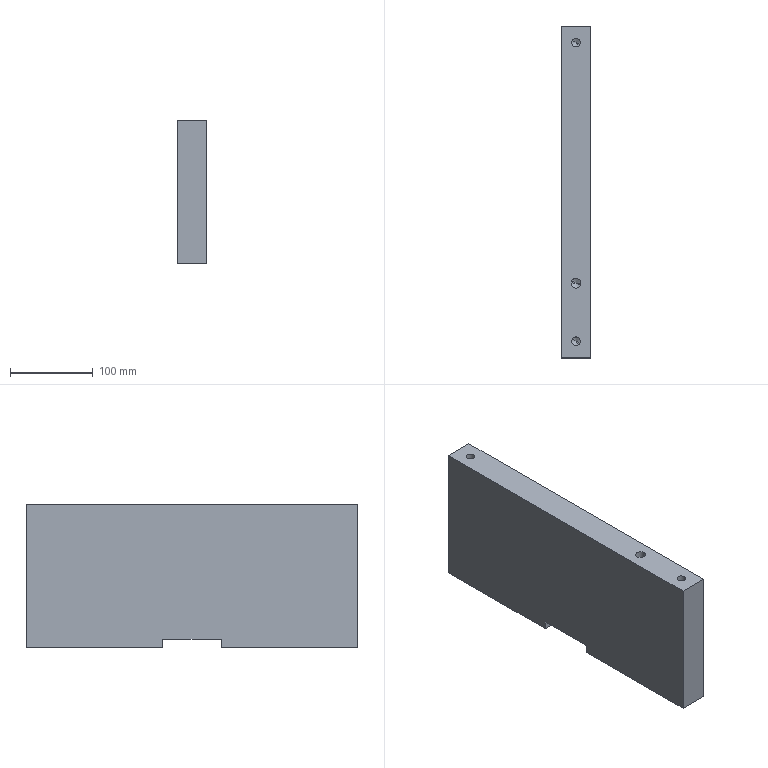Part | CATIA | 1 solid | 42 faces | box 35 x 400 x 173 mm | volume 2372229 mm3 | cone 16 | cylinder 16 | plane 10 | commonest cylinder face diameters 10.2 x10 12 x6
STEP:
#1=CARTESIAN_POINT('',(17.5,200.,-102.));
#2=VERTEX_POINT('',#1);
#3=CARTESIAN_POINT('',(17.5,200.,-275.));
#4=VERTEX_POINT('',#3);
#5=CARTESIAN_POINT('',(17.5,200.,-188.5));
#6=DIRECTION('',(0.,0.,-1.));
#7=VECTOR('',#6,1.);
#8=LINE('',#5,#7);
#9=EDGE_CURVE('',#2,#4,#8,.T.);
#10=ORIENTED_EDGE('',*,*,#9,.T.);
#11=CARTESIAN_POINT('',(-17.5,200.,-275.));
#12=VERTEX_POINT('',#11);
#13=CARTESIAN_POINT('',(0.,200.,-275.));
#14=DIRECTION('',(1.,0.,0.));
#15=VECTOR('',#14,1.);
#16=LINE('',#13,#15);
#17=EDGE_CURVE('',#4,#12,#16,.F.);
#18=ORIENTED_EDGE('',*,*,#17,.T.);
#19=CARTESIAN_POINT('',(-17.5,200.,-102.));
#20=VERTEX_POINT('',#19);
#21=CARTESIAN_POINT('',(-17.5,200.,-188.5));
#22=DIRECTION('',(0.,0.,-1.));
#23=VECTOR('',#22,1.);
#24=LINE('',#21,#23);
#25=EDGE_CURVE('',#20,#12,#24,.T.);
#26=ORIENTED_EDGE('',*,*,#25,.F.);
#27=CARTESIAN_POINT('',(0.,200.,-102.));
#28=DIRECTION('',(1.,0.,0.));
#29=VECTOR('',#28,1.);
#30=LINE('',#27,#29);
#31=EDGE_CURVE('',#20,#2,#30,.T.);
#32=ORIENTED_EDGE('',*,*,#31,.T.);
#33=EDGE_LOOP('',(#10,#18,#26,#32));
#34=FACE_OUTER_BOUND('',#33,.T.);
#35=CARTESIAN_POINT('',(-17.5,200.,0.));
#36=DIRECTION('',(0.,1.,0.));
#37=DIRECTION('',(1.,0.,0.));
#38=AXIS2_PLACEMENT_3D('',#35,#36,#37);
#39=PLANE('',#38);
#40=ADVANCED_FACE('',(#34),#39,.T.);
#41=CARTESIAN_POINT('',(-17.5,-200.,-102.));
#42=VERTEX_POINT('',#41);
#43=CARTESIAN_POINT('',(-17.5,-200.,-275.));
#44=VERTEX_POINT('',#43);
#45=CARTESIAN_POINT('',(-17.5,-200.,-188.5));
#46=DIRECTION('',(0.,0.,-1.));
#47=VECTOR('',#46,1.);
#48=LINE('',#45,#47);
#49=EDGE_CURVE('',#42,#44,#48,.T.);
#50=ORIENTED_EDGE('',*,*,#49,.T.);
#51=CARTESIAN_POINT('',(17.5,-200.,-275.));
#52=VERTEX_POINT('',#51);
#53=CARTESIAN_POINT('',(0.,-200.,-275.));
#54=DIRECTION('',(-1.,0.,0.));
#55=VECTOR('',#54,1.);
#56=LINE('',#53,#55);
#57=EDGE_CURVE('',#44,#52,#56,.F.);
#58=ORIENTED_EDGE('',*,*,#57,.T.);
#59=CARTESIAN_POINT('',(17.5,-200.,-102.));
#60=VERTEX_POINT('',#59);
#61=CARTESIAN_POINT('',(17.5,-200.,-188.5));
#62=DIRECTION('',(0.,0.,-1.));
#63=VECTOR('',#62,1.);
#64=LINE('',#61,#63);
#65=EDGE_CURVE('',#60,#52,#64,.T.);
#66=ORIENTED_EDGE('',*,*,#65,.F.);
#67=CARTESIAN_POINT('',(0.,-200.,-102.));
#68=DIRECTION('',(-1.,0.,0.));
#69=VECTOR('',#68,1.);
#70=LINE('',#67,#69);
#71=EDGE_CURVE('',#60,#42,#70,.T.);
#72=ORIENTED_EDGE('',*,*,#71,.T.);
#73=EDGE_LOOP('',(#50,#58,#66,#72));
#74=FACE_OUTER_BOUND('',#73,.T.);
#75=CARTESIAN_POINT('',(17.5,-200.,0.));
#76=DIRECTION('',(0.,-1.,0.));
#77=DIRECTION('',(-1.,0.,0.));
#78=AXIS2_PLACEMENT_3D('',#75,#76,#77);
#79=PLANE('',#78);
#80=ADVANCED_FACE('',(#74),#79,.T.);
#81=CARTESIAN_POINT('',(-17.5,35.,-275.));
#82=VERTEX_POINT('',#81);
#83=CARTESIAN_POINT('',(-17.5,35.,-265.));
#84=VERTEX_POINT('',#83);
#85=CARTESIAN_POINT('',(-17.5,35.,-270.));
#86=DIRECTION('',(0.,0.,1.));
#87=VECTOR('',#86,1.);
#88=LINE('',#85,#87);
#89=EDGE_CURVE('',#82,#84,#88,.T.);
#90=ORIENTED_EDGE('',*,*,#89,.T.);
#91=CARTESIAN_POINT('',(-17.5,-35.,-265.));
#92=VERTEX_POINT('',#91);
#93=CARTESIAN_POINT('',(-17.5,0.,-265.));
#94=DIRECTION('',(0.,1.,0.));
#95=VECTOR('',#94,1.);
#96=LINE('',#93,#95);
#97=EDGE_CURVE('',#92,#84,#96,.T.);
#98=ORIENTED_EDGE('',*,*,#97,.F.);
#99=CARTESIAN_POINT('',(-17.5,-35.,-275.));
#100=VERTEX_POINT('',#99);
#101=CARTESIAN_POINT('',(-17.5,-35.,-270.));
#102=DIRECTION('',(0.,0.,1.));
#103=VECTOR('',#102,1.);
#104=LINE('',#101,#103);
#105=EDGE_CURVE('',#100,#92,#104,.T.);
#106=ORIENTED_EDGE('',*,*,#105,.F.);
#107=CARTESIAN_POINT('',(-17.5,-117.5,-275.));
#108=DIRECTION('',(0.,-1.,0.));
#109=VECTOR('',#108,1.);
#110=LINE('',#107,#109);
#111=EDGE_CURVE('',#100,#44,#110,.T.);
#112=ORIENTED_EDGE('',*,*,#111,.T.);
#113=ORIENTED_EDGE('',*,*,#49,.F.);
#114=CARTESIAN_POINT('',(-17.5,0.,-102.));
#115=DIRECTION('',(0.,-1.,0.));
#116=VECTOR('',#115,1.);
#117=LINE('',#114,#116);
#118=EDGE_CURVE('',#20,#42,#117,.T.);
#119=ORIENTED_EDGE('',*,*,#118,.F.);
#120=ORIENTED_EDGE('',*,*,#25,.T.);
#121=CARTESIAN_POINT('',(-17.5,117.5,-275.));
#122=DIRECTION('',(0.,-1.,0.));
#123=VECTOR('',#122,1.);
#124=LINE('',#121,#123);
#125=EDGE_CURVE('',#12,#82,#124,.T.);
#126=ORIENTED_EDGE('',*,*,#125,.T.);
#127=EDGE_LOOP('',(#90,#98,#106,#112,#113,#119,#120,#126));
#128=FACE_OUTER_BOUND('',#127,.T.);
#129=CARTESIAN_POINT('',(-17.5,200.,0.));
#130=DIRECTION('',(1.,0.,0.));
#131=DIRECTION('',(0.,-1.,0.));
#132=AXIS2_PLACEMENT_3D('',#129,#130,#131);
#133=PLANE('',#132);
#134=ADVANCED_FACE('',(#128),#133,.F.);
#135=CARTESIAN_POINT('',(17.5,-35.,-275.));
#136=VERTEX_POINT('',#135);
#137=CARTESIAN_POINT('',(17.5,-35.,-265.));
#138=VERTEX_POINT('',#137);
#139=CARTESIAN_POINT('',(17.5,-35.,-270.));
#140=DIRECTION('',(0.,0.,1.));
#141=VECTOR('',#140,1.);
#142=LINE('',#139,#141);
#143=EDGE_CURVE('',#136,#138,#142,.T.);
#144=ORIENTED_EDGE('',*,*,#143,.T.);
#145=CARTESIAN_POINT('',(17.5,35.,-265.));
#146=VERTEX_POINT('',#145);
#147=CARTESIAN_POINT('',(17.5,0.,-265.));
#148=DIRECTION('',(0.,1.,0.));
#149=VECTOR('',#148,1.);
#150=LINE('',#147,#149);
#151=EDGE_CURVE('',#138,#146,#150,.T.);
#152=ORIENTED_EDGE('',*,*,#151,.T.);
#153=CARTESIAN_POINT('',(17.5,35.,-275.));
#154=VERTEX_POINT('',#153);
#155=CARTESIAN_POINT('',(17.5,35.,-270.));
#156=DIRECTION('',(0.,0.,1.));
#157=VECTOR('',#156,1.);
#158=LINE('',#155,#157);
#159=EDGE_CURVE('',#154,#146,#158,.T.);
#160=ORIENTED_EDGE('',*,*,#159,.F.);
#161=CARTESIAN_POINT('',(17.5,117.5,-275.));
#162=DIRECTION('',(0.,1.,0.));
#163=VECTOR('',#162,1.);
#164=LINE('',#161,#163);
#165=EDGE_CURVE('',#154,#4,#164,.T.);
#166=ORIENTED_EDGE('',*,*,#165,.T.);
#167=ORIENTED_EDGE('',*,*,#9,.F.);
#168=CARTESIAN_POINT('',(17.5,0.,-102.));
#169=DIRECTION('',(0.,1.,0.));
#170=VECTOR('',#169,1.);
#171=LINE('',#168,#170);
#172=EDGE_CURVE('',#60,#2,#171,.T.);
#173=ORIENTED_EDGE('',*,*,#172,.F.);
#174=ORIENTED_EDGE('',*,*,#65,.T.);
#175=CARTESIAN_POINT('',(17.5,-117.5,-275.));
#176=DIRECTION('',(0.,1.,0.));
#177=VECTOR('',#176,1.);
#178=LINE('',#175,#177);
#179=EDGE_CURVE('',#52,#136,#178,.T.);
#180=ORIENTED_EDGE('',*,*,#179,.T.);
#181=EDGE_LOOP('',(#144,#152,#160,#166,#167,#173,#174,#180));
#182=FACE_OUTER_BOUND('',#181,.T.);
#183=CARTESIAN_POINT('',(17.5,-200.,0.));
#184=DIRECTION('',(-1.,0.,0.));
#185=DIRECTION('',(0.,1.,0.));
#186=AXIS2_PLACEMENT_3D('',#183,#184,#185);
#187=PLANE('',#186);
#188=ADVANCED_FACE('',(#182),#187,.F.);
#189=ORIENTED_EDGE('',*,*,#151,.F.);
#190=CARTESIAN_POINT('',(0.,-35.,-265.));
#191=DIRECTION('',(1.,0.,0.));
#192=VECTOR('',#191,1.);
#193=LINE('',#190,#192);
#194=EDGE_CURVE('',#138,#92,#193,.F.);
#195=ORIENTED_EDGE('',*,*,#194,.T.);
#196=ORIENTED_EDGE('',*,*,#97,.T.);
#197=CARTESIAN_POINT('',(0.,35.,-265.));
#198=DIRECTION('',(-1.,0.,0.));
#199=VECTOR('',#198,1.);
#200=LINE('',#197,#199);
#201=EDGE_CURVE('',#84,#146,#200,.F.);
#202=ORIENTED_EDGE('',*,*,#201,.T.);
#203=EDGE_LOOP('',(#189,#195,#196,#202));
#204=FACE_OUTER_BOUND('',#203,.T.);
#205=CARTESIAN_POINT('',(0.,0.,-265.));
#206=DIRECTION('',(0.,0.,-1.));
#207=DIRECTION('',(1.,0.,0.));
#208=AXIS2_PLACEMENT_3D('',#205,#206,#207);
#209=PLANE('',#208);
#210=ADVANCED_FACE('',(#204),#209,.T.);
#211=ORIENTED_EDGE('',*,*,#194,.F.);
#212=ORIENTED_EDGE('',*,*,#143,.F.);
#213=CARTESIAN_POINT('',(0.,-35.,-275.));
#214=DIRECTION('',(1.,0.,0.));
#215=VECTOR('',#214,1.);
#216=LINE('',#213,#215);
#217=EDGE_CURVE('',#136,#100,#216,.F.);
#218=ORIENTED_EDGE('',*,*,#217,.T.);
#219=ORIENTED_EDGE('',*,*,#105,.T.);
#220=EDGE_LOOP('',(#211,#212,#218,#219));
#221=FACE_OUTER_BOUND('',#220,.T.);
#222=CARTESIAN_POINT('',(-30.,-35.,-275.));
#223=DIRECTION('',(0.,-1.,0.));
#224=DIRECTION('',(1.,0.,0.));
#225=AXIS2_PLACEMENT_3D('',#222,#223,#224);
#226=PLANE('',#225);
#227=ADVANCED_FACE('',(#221),#226,.F.);
#228=ORIENTED_EDGE('',*,*,#201,.F.);
#229=ORIENTED_EDGE('',*,*,#89,.F.);
#230=CARTESIAN_POINT('',(0.,35.,-275.));
#231=DIRECTION('',(-1.,0.,0.));
#232=VECTOR('',#231,1.);
#233=LINE('',#230,#232);
#234=EDGE_CURVE('',#82,#154,#233,.F.);
#235=ORIENTED_EDGE('',*,*,#234,.T.);
#236=ORIENTED_EDGE('',*,*,#159,.T.);
#237=EDGE_LOOP('',(#228,#229,#235,#236));
#238=FACE_OUTER_BOUND('',#237,.T.);
#239=CARTESIAN_POINT('',(35.,35.,-275.));
#240=DIRECTION('',(0.,1.,0.));
#241=DIRECTION('',(-1.,0.,0.));
#242=AXIS2_PLACEMENT_3D('',#239,#240,#241);
#243=PLANE('',#242);
#244=ADVANCED_FACE('',(#238),#243,.F.);
#245=ORIENTED_EDGE('',*,*,#234,.F.);
#246=ORIENTED_EDGE('',*,*,#125,.F.);
#247=ORIENTED_EDGE('',*,*,#17,.F.);
#248=ORIENTED_EDGE('',*,*,#165,.F.);
#249=EDGE_LOOP('',(#245,#246,#247,#248));
#250=FACE_OUTER_BOUND('',#249,.T.);
#251=CARTESIAN_POINT('',(4.476,177.445,-275.));
#252=VERTEX_POINT('',#251);
#253=CARTESIAN_POINT('',(-4.476,172.555,-275.));
#254=VERTEX_POINT('',#253);
#255=CARTESIAN_POINT('',(0.,175.,-275.));
#256=DIRECTION('',(0.,0.,1.));
#257=AXIS2_PLACEMENT_3D('',#255,#256,$);
#258=CIRCLE('',#257,5.1);
#259=EDGE_CURVE('',#252,#254,#258,.T.);
#260=ORIENTED_EDGE('',*,*,#259,.T.);
#261=CARTESIAN_POINT('',(0.,175.,-275.));
#262=DIRECTION('',(0.,0.,1.));
#263=AXIS2_PLACEMENT_3D('',#261,#262,$);
#264=CIRCLE('',#263,5.1);
#265=EDGE_CURVE('',#254,#252,#264,.T.);
#266=ORIENTED_EDGE('',*,*,#265,.T.);
#267=EDGE_LOOP('',(#260,#266));
#268=FACE_BOUND('',#267,.T.);
#269=CARTESIAN_POINT('',(5.265,112.877,-275.));
#270=VERTEX_POINT('',#269);
#271=CARTESIAN_POINT('',(-5.265,107.123,-275.));
#272=VERTEX_POINT('',#271);
#273=CARTESIAN_POINT('',(0.,110.,-275.));
#274=DIRECTION('',(0.,0.,1.));
#275=AXIS2_PLACEMENT_3D('',#273,#274,$);
#276=CIRCLE('',#275,6.);
#277=EDGE_CURVE('',#270,#272,#276,.T.);
#278=ORIENTED_EDGE('',*,*,#277,.T.);
#279=CARTESIAN_POINT('',(0.,110.,-275.));
#280=DIRECTION('',(0.,0.,1.));
#281=AXIS2_PLACEMENT_3D('',#279,#280,$);
#282=CIRCLE('',#281,6.);
#283=EDGE_CURVE('',#272,#270,#282,.T.);
#284=ORIENTED_EDGE('',*,*,#283,.T.);
#285=EDGE_LOOP('',(#278,#284));
#286=FACE_BOUND('',#285,.T.);
#287=CARTESIAN_POINT('',(0.,0.,-275.));
#288=DIRECTION('',(0.,0.,1.));
#289=DIRECTION('',(1.,0.,0.));
#290=AXIS2_PLACEMENT_3D('',#287,#288,#289);
#291=PLANE('',#290);
#292=ADVANCED_FACE('',(#250,#268,#286),#291,.F.);
#293=ORIENTED_EDGE('',*,*,#217,.F.);
#294=ORIENTED_EDGE('',*,*,#179,.F.);
#295=ORIENTED_EDGE('',*,*,#57,.F.);
#296=ORIENTED_EDGE('',*,*,#111,.F.);
#297=EDGE_LOOP('',(#293,#294,#295,#296));
#298=FACE_OUTER_BOUND('',#297,.T.);
#299=CARTESIAN_POINT('',(4.476,-172.555,-275.));
#300=VERTEX_POINT('',#299);
#301=CARTESIAN_POINT('',(-4.476,-177.445,-275.));
#302=VERTEX_POINT('',#301);
#303=CARTESIAN_POINT('',(0.,-175.,-275.));
#304=DIRECTION('',(0.,0.,1.));
#305=AXIS2_PLACEMENT_3D('',#303,#304,$);
#306=CIRCLE('',#305,5.1);
#307=EDGE_CURVE('',#300,#302,#306,.T.);
#308=ORIENTED_EDGE('',*,*,#307,.T.);
#309=CARTESIAN_POINT('',(0.,-175.,-275.));
#310=DIRECTION('',(0.,0.,1.));
#311=AXIS2_PLACEMENT_3D('',#309,#310,$);
#312=CIRCLE('',#311,5.1);
#313=EDGE_CURVE('',#302,#300,#312,.T.);
#314=ORIENTED_EDGE('',*,*,#313,.T.);
#315=EDGE_LOOP('',(#308,#314));
#316=FACE_BOUND('',#315,.T.);
#317=CARTESIAN_POINT('',(4.476,-57.555,-275.));
#318=VERTEX_POINT('',#317);
#319=CARTESIAN_POINT('',(-4.476,-62.445,-275.));
#320=VERTEX_POINT('',#319);
#321=CARTESIAN_POINT('',(0.,-60.,-275.));
#322=DIRECTION('',(0.,0.,1.));
#323=AXIS2_PLACEMENT_3D('',#321,#322,$);
#324=CIRCLE('',#323,5.1);
#325=EDGE_CURVE('',#318,#320,#324,.T.);
#326=ORIENTED_EDGE('',*,*,#325,.T.);
#327=CARTESIAN_POINT('',(0.,-60.,-275.));
#328=DIRECTION('',(0.,0.,1.));
#329=AXIS2_PLACEMENT_3D('',#327,#328,$);
#330=CIRCLE('',#329,5.1);
#331=EDGE_CURVE('',#320,#318,#330,.T.);
#332=ORIENTED_EDGE('',*,*,#331,.T.);
#333=EDGE_LOOP('',(#326,#332));
#334=FACE_BOUND('',#333,.T.);
#335=CARTESIAN_POINT('',(5.265,-107.123,-275.));
#336=VERTEX_POINT('',#335);
#337=CARTESIAN_POINT('',(-5.265,-112.877,-275.));
#338=VERTEX_POINT('',#337);
#339=CARTESIAN_POINT('',(0.,-110.,-275.));
#340=DIRECTION('',(0.,0.,1.));
#341=AXIS2_PLACEMENT_3D('',#339,#340,$);
#342=CIRCLE('',#341,6.);
#343=EDGE_CURVE('',#336,#338,#342,.T.);
#344=ORIENTED_EDGE('',*,*,#343,.T.);
#345=CARTESIAN_POINT('',(0.,-110.,-275.));
#346=DIRECTION('',(0.,0.,1.));
#347=AXIS2_PLACEMENT_3D('',#345,#346,$);
#348=CIRCLE('',#347,6.);
#349=EDGE_CURVE('',#338,#336,#348,.T.);
#350=ORIENTED_EDGE('',*,*,#349,.T.);
#351=EDGE_LOOP('',(#344,#350));
#352=FACE_BOUND('',#351,.T.);
#353=ADVANCED_FACE('',(#298,#316,#334,#352),#291,.F.);
#354=ORIENTED_EDGE('',*,*,#31,.F.);
#355=ORIENTED_EDGE('',*,*,#118,.T.);
#356=ORIENTED_EDGE('',*,*,#71,.F.);
#357=ORIENTED_EDGE('',*,*,#172,.T.);
#358=EDGE_LOOP('',(#354,#355,#356,#357));
#359=FACE_OUTER_BOUND('',#358,.T.);
#360=CARTESIAN_POINT('',(4.476,-182.445,-102.));
#361=VERTEX_POINT('',#360);
#362=CARTESIAN_POINT('',(-4.476,-177.555,-102.));
#363=VERTEX_POINT('',#362);
#364=CARTESIAN_POINT('',(0.,-180.,-102.));
#365=DIRECTION('',(0.,0.,1.));
#366=AXIS2_PLACEMENT_3D('',#364,#365,$);
#367=CIRCLE('',#366,5.1);
#368=EDGE_CURVE('',#361,#363,#367,.T.);
#369=ORIENTED_EDGE('',*,*,#368,.F.);
#370=CARTESIAN_POINT('',(0.,-180.,-102.));
#371=DIRECTION('',(0.,0.,1.));
#372=AXIS2_PLACEMENT_3D('',#370,#371,$);
#373=CIRCLE('',#372,5.1);
#374=EDGE_CURVE('',#363,#361,#373,.T.);
#375=ORIENTED_EDGE('',*,*,#374,.F.);
#376=EDGE_LOOP('',(#369,#375));
#377=FACE_BOUND('',#376,.T.);
#378=CARTESIAN_POINT('',(4.476,177.555,-102.));
#379=VERTEX_POINT('',#378);
#380=CARTESIAN_POINT('',(-4.476,182.445,-102.));
#381=VERTEX_POINT('',#380);
#382=CARTESIAN_POINT('',(0.,180.,-102.));
#383=DIRECTION('',(0.,0.,1.));
#384=AXIS2_PLACEMENT_3D('',#382,#383,$);
#385=CIRCLE('',#384,5.1);
#386=EDGE_CURVE('',#379,#381,#385,.T.);
#387=ORIENTED_EDGE('',*,*,#386,.F.);
#388=CARTESIAN_POINT('',(0.,180.,-102.));
#389=DIRECTION('',(0.,0.,1.));
#390=AXIS2_PLACEMENT_3D('',#388,#389,$);
#391=CIRCLE('',#390,5.1);
#392=EDGE_CURVE('',#381,#379,#391,.T.);
#393=ORIENTED_EDGE('',*,*,#392,.F.);
#394=EDGE_LOOP('',(#387,#393));
#395=FACE_BOUND('',#394,.T.);
#396=CARTESIAN_POINT('',(5.265,-112.877,-102.));
#397=VERTEX_POINT('',#396);
#398=CARTESIAN_POINT('',(-5.265,-107.123,-102.));
#399=VERTEX_POINT('',#398);
#400=CARTESIAN_POINT('',(0.,-110.,-102.));
#401=DIRECTION('',(0.,0.,1.));
#402=AXIS2_PLACEMENT_3D('',#400,#401,$);
#403=CIRCLE('',#402,6.);
#404=EDGE_CURVE('',#397,#399,#403,.T.);
#405=ORIENTED_EDGE('',*,*,#404,.F.);
#406=CARTESIAN_POINT('',(0.,-110.,-102.));
#407=DIRECTION('',(0.,0.,1.));
#408=AXIS2_PLACEMENT_3D('',#406,#407,$);
#409=CIRCLE('',#408,6.);
#410=EDGE_CURVE('',#399,#397,#409,.T.);
#411=ORIENTED_EDGE('',*,*,#410,.F.);
#412=EDGE_LOOP('',(#405,#411));
#413=FACE_BOUND('',#412,.T.);
#414=CARTESIAN_POINT('',(0.,0.,-102.));
#415=DIRECTION('',(0.,0.,1.));
#416=DIRECTION('',(1.,0.,0.));
#417=AXIS2_PLACEMENT_3D('',#414,#415,#416);
#418=PLANE('',#417);
#419=ADVANCED_FACE('',(#359,#377,#395,#413),#418,.T.);
#420=CARTESIAN_POINT('',(0.,-110.,-135.464));
#421=VERTEX_POINT('',#420);
#422=CARTESIAN_POINT('',(-5.265,-107.123,-132.));
#423=VERTEX_POINT('',#422);
#424=CARTESIAN_POINT('',(-2.633,-108.562,-133.732));
#425=DIRECTION('',(-0.76,0.4152,0.5));
#426=VECTOR('',#425,1.);
#427=LINE('',#424,#426);
#428=EDGE_CURVE('',#421,#423,#427,.T.);
#429=ORIENTED_EDGE('',*,*,#428,.T.);
#430=CARTESIAN_POINT('',(5.265,-112.877,-132.));
#431=VERTEX_POINT('',#430);
#432=CARTESIAN_POINT('',(0.,-110.,-132.));
#433=DIRECTION('',(0.,0.,1.));
#434=AXIS2_PLACEMENT_3D('',#432,#433,$);
#435=CIRCLE('',#434,6.);
#436=EDGE_CURVE('',#431,#423,#435,.F.);
#437=ORIENTED_EDGE('',*,*,#436,.F.);
#438=CARTESIAN_POINT('',(2.633,-111.438,-133.732));
#439=DIRECTION('',(0.76,-0.4152,0.5));
#440=VECTOR('',#439,1.);
#441=LINE('',#438,#440);
#442=EDGE_CURVE('',#421,#431,#441,.T.);
#443=ORIENTED_EDGE('',*,*,#442,.F.);
#444=EDGE_LOOP('',(#429,#437,#443));
#445=FACE_OUTER_BOUND('',#444,.T.);
#446=CARTESIAN_POINT('',(0.,-110.,-135.464));
#447=DIRECTION('',(0.,0.,1.));
#448=DIRECTION('',(0.8776,-0.4794,0.));
#449=AXIS2_PLACEMENT_3D('',#446,#447,#448);
#450=CONICAL_SURFACE('',#449,0.,1.047);
#451=ADVANCED_FACE('',(#445),#450,.F.);
#452=ORIENTED_EDGE('',*,*,#442,.T.);
#453=CARTESIAN_POINT('',(0.,-110.,-132.));
#454=DIRECTION('',(0.,0.,1.));
#455=AXIS2_PLACEMENT_3D('',#453,#454,$);
#456=CIRCLE('',#455,6.);
#457=EDGE_CURVE('',#423,#431,#456,.F.);
#458=ORIENTED_EDGE('',*,*,#457,.F.);
#459=ORIENTED_EDGE('',*,*,#428,.F.);
#460=EDGE_LOOP('',(#452,#458,#459));
#461=FACE_OUTER_BOUND('',#460,.T.);
#462=ADVANCED_FACE('',(#461),#450,.F.);
#463=ORIENTED_EDGE('',*,*,#410,.T.);
#464=CARTESIAN_POINT('',(5.265,-112.877,-116.8));
#465=DIRECTION('',(0.,0.,-1.));
#466=VECTOR('',#465,1.);
#467=LINE('',#464,#466);
#468=EDGE_CURVE('',#431,#397,#467,.F.);
#469=ORIENTED_EDGE('',*,*,#468,.F.);
#470=ORIENTED_EDGE('',*,*,#436,.T.);
#471=CARTESIAN_POINT('',(-5.265,-107.123,-116.8));
#472=DIRECTION('',(0.,0.,-1.));
#473=VECTOR('',#472,1.);
#474=LINE('',#471,#473);
#475=EDGE_CURVE('',#423,#399,#474,.F.);
#476=ORIENTED_EDGE('',*,*,#475,.T.);
#477=EDGE_LOOP('',(#463,#469,#470,#476));
#478=FACE_OUTER_BOUND('',#477,.T.);
#479=CARTESIAN_POINT('',(0.,-110.,-102.1));
#480=DIRECTION('',(0.,0.,-1.));
#481=DIRECTION('',(0.8776,-0.4794,0.));
#482=AXIS2_PLACEMENT_3D('',#479,#480,#481);
#483=CYLINDRICAL_SURFACE('',#482,6.);
#484=ADVANCED_FACE('',(#478),#483,.F.);
#485=ORIENTED_EDGE('',*,*,#404,.T.);
#486=ORIENTED_EDGE('',*,*,#475,.F.);
#487=ORIENTED_EDGE('',*,*,#457,.T.);
#488=ORIENTED_EDGE('',*,*,#468,.T.);
#489=EDGE_LOOP('',(#485,#486,#487,#488));
#490=FACE_OUTER_BOUND('',#489,.T.);
#491=ADVANCED_FACE('',(#490),#483,.F.);
#492=CARTESIAN_POINT('',(0.,110.,-241.536));
#493=VERTEX_POINT('',#492);
#494=CARTESIAN_POINT('',(-5.265,107.123,-245.));
#495=VERTEX_POINT('',#494);
#496=CARTESIAN_POINT('',(-2.633,108.562,-243.268));
#497=DIRECTION('',(-0.76,-0.4152,-0.5));
#498=VECTOR('',#497,1.);
#499=LINE('',#496,#498);
#500=EDGE_CURVE('',#493,#495,#499,.T.);
#501=ORIENTED_EDGE('',*,*,#500,.T.);
#502=CARTESIAN_POINT('',(5.265,112.877,-245.));
#503=VERTEX_POINT('',#502);
#504=CARTESIAN_POINT('',(0.,110.,-245.));
#505=DIRECTION('',(0.,0.,-1.));
#506=AXIS2_PLACEMENT_3D('',#504,#505,$);
#507=CIRCLE('',#506,6.);
#508=EDGE_CURVE('',#503,#495,#507,.F.);
#509=ORIENTED_EDGE('',*,*,#508,.F.);
#510=CARTESIAN_POINT('',(2.633,111.438,-243.268));
#511=DIRECTION('',(0.76,0.4152,-0.5));
#512=VECTOR('',#511,1.);
#513=LINE('',#510,#512);
#514=EDGE_CURVE('',#493,#503,#513,.T.);
#515=ORIENTED_EDGE('',*,*,#514,.F.);
#516=EDGE_LOOP('',(#501,#509,#515));
#517=FACE_OUTER_BOUND('',#516,.T.);
#518=CARTESIAN_POINT('',(0.,110.,-241.536));
#519=DIRECTION('',(0.,0.,-1.));
#520=DIRECTION('',(0.8776,0.4794,0.));
#521=AXIS2_PLACEMENT_3D('',#518,#519,#520);
#522=CONICAL_SURFACE('',#521,0.,1.047);
#523=ADVANCED_FACE('',(#517),#522,.F.);
#524=ORIENTED_EDGE('',*,*,#514,.T.);
#525=CARTESIAN_POINT('',(0.,110.,-245.));
#526=DIRECTION('',(0.,0.,-1.));
#527=AXIS2_PLACEMENT_3D('',#525,#526,$);
#528=CIRCLE('',#527,6.);
#529=EDGE_CURVE('',#495,#503,#528,.F.);
#530=ORIENTED_EDGE('',*,*,#529,.F.);
#531=ORIENTED_EDGE('',*,*,#500,.F.);
#532=EDGE_LOOP('',(#524,#530,#531));
#533=FACE_OUTER_BOUND('',#532,.T.);
#534=ADVANCED_FACE('',(#533),#522,.F.);
#535=ORIENTED_EDGE('',*,*,#277,.F.);
#536=CARTESIAN_POINT('',(5.265,112.877,-260.2));
#537=DIRECTION('',(0.,0.,1.));
#538=VECTOR('',#537,1.);
#539=LINE('',#536,#538);
#540=EDGE_CURVE('',#503,#270,#539,.F.);
#541=ORIENTED_EDGE('',*,*,#540,.F.);
#542=ORIENTED_EDGE('',*,*,#508,.T.);
#543=CARTESIAN_POINT('',(-5.265,107.123,-260.2));
#544=DIRECTION('',(0.,0.,1.));
#545=VECTOR('',#544,1.);
#546=LINE('',#543,#545);
#547=EDGE_CURVE('',#495,#272,#546,.F.);
#548=ORIENTED_EDGE('',*,*,#547,.T.);
#549=EDGE_LOOP('',(#535,#541,#542,#548));
#550=FACE_OUTER_BOUND('',#549,.T.);
#551=CARTESIAN_POINT('',(0.,110.,-274.9));
#552=DIRECTION('',(0.,0.,1.));
#553=DIRECTION('',(0.8776,0.4794,0.));
#554=AXIS2_PLACEMENT_3D('',#551,#552,#553);
#555=CYLINDRICAL_SURFACE('',#554,6.);
#556=ADVANCED_FACE('',(#550),#555,.F.);
#557=ORIENTED_EDGE('',*,*,#283,.F.);
#558=ORIENTED_EDGE('',*,*,#547,.F.);
#559=ORIENTED_EDGE('',*,*,#529,.T.);
#560=ORIENTED_EDGE('',*,*,#540,.T.);
#561=EDGE_LOOP('',(#557,#558,#559,#560));
#562=FACE_OUTER_BOUND('',#561,.T.);
#563=ADVANCED_FACE('',(#562),#555,.F.);
#564=CARTESIAN_POINT('',(0.,-60.,-237.056));
#565=VERTEX_POINT('',#564);
#566=CARTESIAN_POINT('',(-4.476,-62.445,-240.));
#567=VERTEX_POINT('',#566);
#568=CARTESIAN_POINT('',(-2.238,-61.223,-238.528));
#569=DIRECTION('',(-0.76,-0.4152,-0.5));
#570=VECTOR('',#569,1.);
#571=LINE('',#568,#570);
#572=EDGE_CURVE('',#565,#567,#571,.T.);
#573=ORIENTED_EDGE('',*,*,#572,.T.);
#574=CARTESIAN_POINT('',(4.476,-57.555,-240.));
#575=VERTEX_POINT('',#574);
#576=CARTESIAN_POINT('',(0.,-60.,-240.));
#577=DIRECTION('',(0.,0.,-1.));
#578=AXIS2_PLACEMENT_3D('',#576,#577,$);
#579=CIRCLE('',#578,5.1);
#580=EDGE_CURVE('',#575,#567,#579,.F.);
#581=ORIENTED_EDGE('',*,*,#580,.F.);
#582=CARTESIAN_POINT('',(2.238,-58.777,-238.528));
#583=DIRECTION('',(0.76,0.4152,-0.5));
#584=VECTOR('',#583,1.);
#585=LINE('',#582,#584);
#586=EDGE_CURVE('',#565,#575,#585,.T.);
#587=ORIENTED_EDGE('',*,*,#586,.F.);
#588=EDGE_LOOP('',(#573,#581,#587));
#589=FACE_OUTER_BOUND('',#588,.T.);
#590=CARTESIAN_POINT('',(0.,-60.,-237.056));
#591=DIRECTION('',(0.,0.,-1.));
#592=DIRECTION('',(0.8776,0.4794,0.));
#593=AXIS2_PLACEMENT_3D('',#590,#591,#592);
#594=CONICAL_SURFACE('',#593,0.,1.047);
#595=ADVANCED_FACE('',(#589),#594,.F.);
#596=ORIENTED_EDGE('',*,*,#586,.T.);
#597=CARTESIAN_POINT('',(0.,-60.,-240.));
#598=DIRECTION('',(0.,0.,-1.));
#599=AXIS2_PLACEMENT_3D('',#597,#598,$);
#600=CIRCLE('',#599,5.1);
#601=EDGE_CURVE('',#567,#575,#600,.F.);
#602=ORIENTED_EDGE('',*,*,#601,.F.);
#603=ORIENTED_EDGE('',*,*,#572,.F.);
#604=EDGE_LOOP('',(#596,#602,#603));
#605=FACE_OUTER_BOUND('',#604,.T.);
#606=ADVANCED_FACE('',(#605),#594,.F.);
#607=ORIENTED_EDGE('',*,*,#325,.F.);
#608=CARTESIAN_POINT('',(4.476,-57.555,-257.7));
#609=DIRECTION('',(0.,0.,1.));
#610=VECTOR('',#609,1.);
#611=LINE('',#608,#610);
#612=EDGE_CURVE('',#575,#318,#611,.F.);
#613=ORIENTED_EDGE('',*,*,#612,.F.);
#614=ORIENTED_EDGE('',*,*,#580,.T.);
#615=CARTESIAN_POINT('',(-4.476,-62.445,-257.7));
#616=DIRECTION('',(0.,0.,1.));
#617=VECTOR('',#616,1.);
#618=LINE('',#615,#617);
#619=EDGE_CURVE('',#567,#320,#618,.F.);
#620=ORIENTED_EDGE('',*,*,#619,.T.);
#621=EDGE_LOOP('',(#607,#613,#614,#620));
#622=FACE_OUTER_BOUND('',#621,.T.);
#623=CARTESIAN_POINT('',(0.,-60.,-274.9));
#624=DIRECTION('',(0.,0.,1.));
#625=DIRECTION('',(0.8776,0.4794,0.));
#626=AXIS2_PLACEMENT_3D('',#623,#624,#625);
#627=CYLINDRICAL_SURFACE('',#626,5.1);
#628=ADVANCED_FACE('',(#622),#627,.F.);
#629=ORIENTED_EDGE('',*,*,#331,.F.);
#630=ORIENTED_EDGE('',*,*,#619,.F.);
#631=ORIENTED_EDGE('',*,*,#601,.T.);
#632=ORIENTED_EDGE('',*,*,#612,.T.);
#633=EDGE_LOOP('',(#629,#630,#631,#632));
#634=FACE_OUTER_BOUND('',#633,.T.);
#635=ADVANCED_FACE('',(#634),#627,.F.);
#636=CARTESIAN_POINT('',(0.,-180.,-139.944));
#637=VERTEX_POINT('',#636);
#638=CARTESIAN_POINT('',(-4.476,-177.555,-137.));
#639=VERTEX_POINT('',#638);
#640=CARTESIAN_POINT('',(-2.238,-178.777,-138.472));
#641=DIRECTION('',(-0.76,0.4152,0.5));
#642=VECTOR('',#641,1.);
#643=LINE('',#640,#642);
#644=EDGE_CURVE('',#637,#639,#643,.T.);
#645=ORIENTED_EDGE('',*,*,#644,.T.);
#646=CARTESIAN_POINT('',(4.476,-182.445,-137.));
#647=VERTEX_POINT('',#646);
#648=CARTESIAN_POINT('',(0.,-180.,-137.));
#649=DIRECTION('',(0.,0.,1.));
#650=AXIS2_PLACEMENT_3D('',#648,#649,$);
#651=CIRCLE('',#650,5.1);
#652=EDGE_CURVE('',#647,#639,#651,.F.);
#653=ORIENTED_EDGE('',*,*,#652,.F.);
#654=CARTESIAN_POINT('',(2.238,-181.223,-138.472));
#655=DIRECTION('',(0.76,-0.4152,0.5));
#656=VECTOR('',#655,1.);
#657=LINE('',#654,#656);
#658=EDGE_CURVE('',#637,#647,#657,.T.);
#659=ORIENTED_EDGE('',*,*,#658,.F.);
#660=EDGE_LOOP('',(#645,#653,#659));
#661=FACE_OUTER_BOUND('',#660,.T.);
#662=CARTESIAN_POINT('',(0.,-180.,-139.944));
#663=DIRECTION('',(0.,0.,1.));
#664=DIRECTION('',(0.8776,-0.4794,0.));
#665=AXIS2_PLACEMENT_3D('',#662,#663,#664);
#666=CONICAL_SURFACE('',#665,0.,1.047);
#667=ADVANCED_FACE('',(#661),#666,.F.);
#668=ORIENTED_EDGE('',*,*,#658,.T.);
#669=CARTESIAN_POINT('',(0.,-180.,-137.));
#670=DIRECTION('',(0.,0.,1.));
#671=AXIS2_PLACEMENT_3D('',#669,#670,$);
#672=CIRCLE('',#671,5.1);
#673=EDGE_CURVE('',#639,#647,#672,.F.);
#674=ORIENTED_EDGE('',*,*,#673,.F.);
#675=ORIENTED_EDGE('',*,*,#644,.F.);
#676=EDGE_LOOP('',(#668,#674,#675));
#677=FACE_OUTER_BOUND('',#676,.T.);
#678=ADVANCED_FACE('',(#677),#666,.F.);
#679=ORIENTED_EDGE('',*,*,#374,.T.);
#680=CARTESIAN_POINT('',(4.476,-182.445,-119.3));
#681=DIRECTION('',(0.,0.,-1.));
#682=VECTOR('',#681,1.);
#683=LINE('',#680,#682);
#684=EDGE_CURVE('',#647,#361,#683,.F.);
#685=ORIENTED_EDGE('',*,*,#684,.F.);
#686=ORIENTED_EDGE('',*,*,#652,.T.);
#687=CARTESIAN_POINT('',(-4.476,-177.555,-119.3));
#688=DIRECTION('',(0.,0.,-1.));
#689=VECTOR('',#688,1.);
#690=LINE('',#687,#689);
#691=EDGE_CURVE('',#639,#363,#690,.F.);
#692=ORIENTED_EDGE('',*,*,#691,.T.);
#693=EDGE_LOOP('',(#679,#685,#686,#692));
#694=FACE_OUTER_BOUND('',#693,.T.);
#695=CARTESIAN_POINT('',(0.,-180.,-102.1));
#696=DIRECTION('',(0.,0.,-1.));
#697=DIRECTION('',(0.8776,-0.4794,0.));
#698=AXIS2_PLACEMENT_3D('',#695,#696,#697);
#699=CYLINDRICAL_SURFACE('',#698,5.1);
#700=ADVANCED_FACE('',(#694),#699,.F.);
#701=ORIENTED_EDGE('',*,*,#368,.T.);
#702=ORIENTED_EDGE('',*,*,#691,.F.);
#703=ORIENTED_EDGE('',*,*,#673,.T.);
#704=ORIENTED_EDGE('',*,*,#684,.T.);
#705=EDGE_LOOP('',(#701,#702,#703,#704));
#706=FACE_OUTER_BOUND('',#705,.T.);
#707=ADVANCED_FACE('',(#706),#699,.F.);
#708=CARTESIAN_POINT('',(0.,-175.,-237.056));
#709=VERTEX_POINT('',#708);
#710=CARTESIAN_POINT('',(-4.476,-177.445,-240.));
#711=VERTEX_POINT('',#710);
#712=CARTESIAN_POINT('',(-2.238,-176.223,-238.528));
#713=DIRECTION('',(-0.76,-0.4152,-0.5));
#714=VECTOR('',#713,1.);
#715=LINE('',#712,#714);
#716=EDGE_CURVE('',#709,#711,#715,.T.);
#717=ORIENTED_EDGE('',*,*,#716,.T.);
#718=CARTESIAN_POINT('',(4.476,-172.555,-240.));
#719=VERTEX_POINT('',#718);
#720=CARTESIAN_POINT('',(0.,-175.,-240.));
#721=DIRECTION('',(0.,0.,-1.));
#722=AXIS2_PLACEMENT_3D('',#720,#721,$);
#723=CIRCLE('',#722,5.1);
#724=EDGE_CURVE('',#719,#711,#723,.F.);
#725=ORIENTED_EDGE('',*,*,#724,.F.);
#726=CARTESIAN_POINT('',(2.238,-173.777,-238.528));
#727=DIRECTION('',(0.76,0.4152,-0.5));
#728=VECTOR('',#727,1.);
#729=LINE('',#726,#728);
#730=EDGE_CURVE('',#709,#719,#729,.T.);
#731=ORIENTED_EDGE('',*,*,#730,.F.);
#732=EDGE_LOOP('',(#717,#725,#731));
#733=FACE_OUTER_BOUND('',#732,.T.);
#734=CARTESIAN_POINT('',(0.,-175.,-237.056));
#735=DIRECTION('',(0.,0.,-1.));
#736=DIRECTION('',(0.8776,0.4794,0.));
#737=AXIS2_PLACEMENT_3D('',#734,#735,#736);
#738=CONICAL_SURFACE('',#737,0.,1.047);
#739=ADVANCED_FACE('',(#733),#738,.F.);
#740=ORIENTED_EDGE('',*,*,#730,.T.);
#741=CARTESIAN_POINT('',(0.,-175.,-240.));
#742=DIRECTION('',(0.,0.,-1.));
#743=AXIS2_PLACEMENT_3D('',#741,#742,$);
#744=CIRCLE('',#743,5.1);
#745=EDGE_CURVE('',#711,#719,#744,.F.);
#746=ORIENTED_EDGE('',*,*,#745,.F.);
#747=ORIENTED_EDGE('',*,*,#716,.F.);
#748=EDGE_LOOP('',(#740,#746,#747));
#749=FACE_OUTER_BOUND('',#748,.T.);
#750=ADVANCED_FACE('',(#749),#738,.F.);
#751=ORIENTED_EDGE('',*,*,#307,.F.);
#752=CARTESIAN_POINT('',(4.476,-172.555,-257.7));
#753=DIRECTION('',(0.,0.,1.));
#754=VECTOR('',#753,1.);
#755=LINE('',#752,#754);
#756=EDGE_CURVE('',#719,#300,#755,.F.);
#757=ORIENTED_EDGE('',*,*,#756,.F.);
#758=ORIENTED_EDGE('',*,*,#724,.T.);
#759=CARTESIAN_POINT('',(-4.476,-177.445,-257.7));
#760=DIRECTION('',(0.,0.,1.));
#761=VECTOR('',#760,1.);
#762=LINE('',#759,#761);
#763=EDGE_CURVE('',#711,#302,#762,.F.);
#764=ORIENTED_EDGE('',*,*,#763,.T.);
#765=EDGE_LOOP('',(#751,#757,#758,#764));
#766=FACE_OUTER_BOUND('',#765,.T.);
#767=CARTESIAN_POINT('',(0.,-175.,-274.9));
#768=DIRECTION('',(0.,0.,1.));
#769=DIRECTION('',(0.8776,0.4794,0.));
#770=AXIS2_PLACEMENT_3D('',#767,#768,#769);
#771=CYLINDRICAL_SURFACE('',#770,5.1);
#772=ADVANCED_FACE('',(#766),#771,.F.);
#773=ORIENTED_EDGE('',*,*,#313,.F.);
#774=ORIENTED_EDGE('',*,*,#763,.F.);
#775=ORIENTED_EDGE('',*,*,#745,.T.);
#776=ORIENTED_EDGE('',*,*,#756,.T.);
#777=EDGE_LOOP('',(#773,#774,#775,#776));
#778=FACE_OUTER_BOUND('',#777,.T.);
#779=ADVANCED_FACE('',(#778),#771,.F.);
#780=CARTESIAN_POINT('',(0.,180.,-139.944));
#781=VERTEX_POINT('',#780);
#782=CARTESIAN_POINT('',(-4.476,182.445,-137.));
#783=VERTEX_POINT('',#782);
#784=CARTESIAN_POINT('',(-2.238,181.223,-138.472));
#785=DIRECTION('',(-0.76,0.4152,0.5));
#786=VECTOR('',#785,1.);
#787=LINE('',#784,#786);
#788=EDGE_CURVE('',#781,#783,#787,.T.);
#789=ORIENTED_EDGE('',*,*,#788,.T.);
#790=CARTESIAN_POINT('',(4.476,177.555,-137.));
#791=VERTEX_POINT('',#790);
#792=CARTESIAN_POINT('',(0.,180.,-137.));
#793=DIRECTION('',(0.,0.,1.));
#794=AXIS2_PLACEMENT_3D('',#792,#793,$);
#795=CIRCLE('',#794,5.1);
#796=EDGE_CURVE('',#791,#783,#795,.F.);
#797=ORIENTED_EDGE('',*,*,#796,.F.);
#798=CARTESIAN_POINT('',(2.238,178.777,-138.472));
#799=DIRECTION('',(0.76,-0.4152,0.5));
#800=VECTOR('',#799,1.);
#801=LINE('',#798,#800);
#802=EDGE_CURVE('',#781,#791,#801,.T.);
#803=ORIENTED_EDGE('',*,*,#802,.F.);
#804=EDGE_LOOP('',(#789,#797,#803));
#805=FACE_OUTER_BOUND('',#804,.T.);
#806=CARTESIAN_POINT('',(0.,180.,-139.944));
#807=DIRECTION('',(0.,0.,1.));
#808=DIRECTION('',(0.8776,-0.4794,0.));
#809=AXIS2_PLACEMENT_3D('',#806,#807,#808);
#810=CONICAL_SURFACE('',#809,0.,1.047);
#811=ADVANCED_FACE('',(#805),#810,.F.);
#812=ORIENTED_EDGE('',*,*,#802,.T.);
#813=CARTESIAN_POINT('',(0.,180.,-137.));
#814=DIRECTION('',(0.,0.,1.));
#815=AXIS2_PLACEMENT_3D('',#813,#814,$);
#816=CIRCLE('',#815,5.1);
#817=EDGE_CURVE('',#783,#791,#816,.F.);
#818=ORIENTED_EDGE('',*,*,#817,.F.);
#819=ORIENTED_EDGE('',*,*,#788,.F.);
#820=EDGE_LOOP('',(#812,#818,#819));
#821=FACE_OUTER_BOUND('',#820,.T.);
#822=ADVANCED_FACE('',(#821),#810,.F.);
#823=ORIENTED_EDGE('',*,*,#392,.T.);
#824=CARTESIAN_POINT('',(4.476,177.555,-119.3));
#825=DIRECTION('',(0.,0.,-1.));
#826=VECTOR('',#825,1.);
#827=LINE('',#824,#826);
#828=EDGE_CURVE('',#791,#379,#827,.F.);
#829=ORIENTED_EDGE('',*,*,#828,.F.);
#830=ORIENTED_EDGE('',*,*,#796,.T.);
#831=CARTESIAN_POINT('',(-4.476,182.445,-119.3));
#832=DIRECTION('',(0.,0.,-1.));
#833=VECTOR('',#832,1.);
#834=LINE('',#831,#833);
#835=EDGE_CURVE('',#783,#381,#834,.F.);
#836=ORIENTED_EDGE('',*,*,#835,.T.);
#837=EDGE_LOOP('',(#823,#829,#830,#836));
#838=FACE_OUTER_BOUND('',#837,.T.);
#839=CARTESIAN_POINT('',(0.,180.,-102.1));
#840=DIRECTION('',(0.,0.,-1.));
#841=DIRECTION('',(0.8776,-0.4794,0.));
#842=AXIS2_PLACEMENT_3D('',#839,#840,#841);
#843=CYLINDRICAL_SURFACE('',#842,5.1);
#844=ADVANCED_FACE('',(#838),#843,.F.);
#845=ORIENTED_EDGE('',*,*,#386,.T.);
#846=ORIENTED_EDGE('',*,*,#835,.F.);
#847=ORIENTED_EDGE('',*,*,#817,.T.);
#848=ORIENTED_EDGE('',*,*,#828,.T.);
#849=EDGE_LOOP('',(#845,#846,#847,#848));
#850=FACE_OUTER_BOUND('',#849,.T.);
#851=ADVANCED_FACE('',(#850),#843,.F.);
#852=CARTESIAN_POINT('',(0.,-110.,-241.536));
#853=VERTEX_POINT('',#852);
#854=CARTESIAN_POINT('',(-5.265,-112.877,-245.));
#855=VERTEX_POINT('',#854);
#856=CARTESIAN_POINT('',(-2.633,-111.438,-243.268));
#857=DIRECTION('',(-0.76,-0.4152,-0.5));
#858=VECTOR('',#857,1.);
#859=LINE('',#856,#858);
#860=EDGE_CURVE('',#853,#855,#859,.T.);
#861=ORIENTED_EDGE('',*,*,#860,.T.);
#862=CARTESIAN_POINT('',(5.265,-107.123,-245.));
#863=VERTEX_POINT('',#862);
#864=CARTESIAN_POINT('',(0.,-110.,-245.));
#865=DIRECTION('',(0.,0.,-1.));
#866=AXIS2_PLACEMENT_3D('',#864,#865,$);
#867=CIRCLE('',#866,6.);
#868=EDGE_CURVE('',#863,#855,#867,.F.);
#869=ORIENTED_EDGE('',*,*,#868,.F.);
#870=CARTESIAN_POINT('',(2.633,-108.562,-243.268));
#871=DIRECTION('',(0.76,0.4152,-0.5));
#872=VECTOR('',#871,1.);
#873=LINE('',#870,#872);
#874=EDGE_CURVE('',#853,#863,#873,.T.);
#875=ORIENTED_EDGE('',*,*,#874,.F.);
#876=EDGE_LOOP('',(#861,#869,#875));
#877=FACE_OUTER_BOUND('',#876,.T.);
#878=CARTESIAN_POINT('',(0.,-110.,-241.536));
#879=DIRECTION('',(0.,0.,-1.));
#880=DIRECTION('',(0.8776,0.4794,0.));
#881=AXIS2_PLACEMENT_3D('',#878,#879,#880);
#882=CONICAL_SURFACE('',#881,0.,1.047);
#883=ADVANCED_FACE('',(#877),#882,.F.);
#884=ORIENTED_EDGE('',*,*,#874,.T.);
#885=CARTESIAN_POINT('',(0.,-110.,-245.));
#886=DIRECTION('',(0.,0.,-1.));
#887=AXIS2_PLACEMENT_3D('',#885,#886,$);
#888=CIRCLE('',#887,6.);
#889=EDGE_CURVE('',#855,#863,#888,.F.);
#890=ORIENTED_EDGE('',*,*,#889,.F.);
#891=ORIENTED_EDGE('',*,*,#860,.F.);
#892=EDGE_LOOP('',(#884,#890,#891));
#893=FACE_OUTER_BOUND('',#892,.T.);
#894=ADVANCED_FACE('',(#893),#882,.F.);
#895=ORIENTED_EDGE('',*,*,#343,.F.);
#896=CARTESIAN_POINT('',(5.265,-107.123,-260.2));
#897=DIRECTION('',(0.,0.,1.));
#898=VECTOR('',#897,1.);
#899=LINE('',#896,#898);
#900=EDGE_CURVE('',#863,#336,#899,.F.);
#901=ORIENTED_EDGE('',*,*,#900,.F.);
#902=ORIENTED_EDGE('',*,*,#868,.T.);
#903=CARTESIAN_POINT('',(-5.265,-112.877,-260.2));
#904=DIRECTION('',(0.,0.,1.));
#905=VECTOR('',#904,1.);
#906=LINE('',#903,#905);
#907=EDGE_CURVE('',#855,#338,#906,.F.);
#908=ORIENTED_EDGE('',*,*,#907,.T.);
#909=EDGE_LOOP('',(#895,#901,#902,#908));
#910=FACE_OUTER_BOUND('',#909,.T.);
#911=CARTESIAN_POINT('',(0.,-110.,-274.9));
#912=DIRECTION('',(0.,0.,1.));
#913=DIRECTION('',(0.8776,0.4794,0.));
#914=AXIS2_PLACEMENT_3D('',#911,#912,#913);
#915=CYLINDRICAL_SURFACE('',#914,6.);
#916=ADVANCED_FACE('',(#910),#915,.F.);
#917=ORIENTED_EDGE('',*,*,#349,.F.);
#918=ORIENTED_EDGE('',*,*,#907,.F.);
#919=ORIENTED_EDGE('',*,*,#889,.T.);
#920=ORIENTED_EDGE('',*,*,#900,.T.);
#921=EDGE_LOOP('',(#917,#918,#919,#920));
#922=FACE_OUTER_BOUND('',#921,.T.);
#923=ADVANCED_FACE('',(#922),#915,.F.);
#924=CARTESIAN_POINT('',(0.,175.,-237.056));
#925=VERTEX_POINT('',#924);
#926=CARTESIAN_POINT('',(-4.476,172.555,-240.));
#927=VERTEX_POINT('',#926);
#928=CARTESIAN_POINT('',(-2.238,173.777,-238.528));
#929=DIRECTION('',(-0.76,-0.4152,-0.5));
#930=VECTOR('',#929,1.);
#931=LINE('',#928,#930);
#932=EDGE_CURVE('',#925,#927,#931,.T.);
#933=ORIENTED_EDGE('',*,*,#932,.T.);
#934=CARTESIAN_POINT('',(4.476,177.445,-240.));
#935=VERTEX_POINT('',#934);
#936=CARTESIAN_POINT('',(0.,175.,-240.));
#937=DIRECTION('',(0.,0.,-1.));
#938=AXIS2_PLACEMENT_3D('',#936,#937,$);
#939=CIRCLE('',#938,5.1);
#940=EDGE_CURVE('',#935,#927,#939,.F.);
#941=ORIENTED_EDGE('',*,*,#940,.F.);
#942=CARTESIAN_POINT('',(2.238,176.223,-238.528));
#943=DIRECTION('',(0.76,0.4152,-0.5));
#944=VECTOR('',#943,1.);
#945=LINE('',#942,#944);
#946=EDGE_CURVE('',#925,#935,#945,.T.);
#947=ORIENTED_EDGE('',*,*,#946,.F.);
#948=EDGE_LOOP('',(#933,#941,#947));
#949=FACE_OUTER_BOUND('',#948,.T.);
#950=CARTESIAN_POINT('',(0.,175.,-237.056));
#951=DIRECTION('',(0.,0.,-1.));
#952=DIRECTION('',(0.8776,0.4794,0.));
#953=AXIS2_PLACEMENT_3D('',#950,#951,#952);
#954=CONICAL_SURFACE('',#953,0.,1.047);
#955=ADVANCED_FACE('',(#949),#954,.F.);
#956=ORIENTED_EDGE('',*,*,#946,.T.);
#957=CARTESIAN_POINT('',(0.,175.,-240.));
#958=DIRECTION('',(0.,0.,-1.));
#959=AXIS2_PLACEMENT_3D('',#957,#958,$);
#960=CIRCLE('',#959,5.1);
#961=EDGE_CURVE('',#927,#935,#960,.F.);
#962=ORIENTED_EDGE('',*,*,#961,.F.);
#963=ORIENTED_EDGE('',*,*,#932,.F.);
#964=EDGE_LOOP('',(#956,#962,#963));
#965=FACE_OUTER_BOUND('',#964,.T.);
#966=ADVANCED_FACE('',(#965),#954,.F.);
#967=ORIENTED_EDGE('',*,*,#259,.F.);
#968=CARTESIAN_POINT('',(4.476,177.445,-257.7));
#969=DIRECTION('',(0.,0.,1.));
#970=VECTOR('',#969,1.);
#971=LINE('',#968,#970);
#972=EDGE_CURVE('',#935,#252,#971,.F.);
#973=ORIENTED_EDGE('',*,*,#972,.F.);
#974=ORIENTED_EDGE('',*,*,#940,.T.);
#975=CARTESIAN_POINT('',(-4.476,172.555,-257.7));
#976=DIRECTION('',(0.,0.,1.));
#977=VECTOR('',#976,1.);
#978=LINE('',#975,#977);
#979=EDGE_CURVE('',#927,#254,#978,.F.);
#980=ORIENTED_EDGE('',*,*,#979,.T.);
#981=EDGE_LOOP('',(#967,#973,#974,#980));
#982=FACE_OUTER_BOUND('',#981,.T.);
#983=CARTESIAN_POINT('',(0.,175.,-274.9));
#984=DIRECTION('',(0.,0.,1.));
#985=DIRECTION('',(0.8776,0.4794,0.));
#986=AXIS2_PLACEMENT_3D('',#983,#984,#985);
#987=CYLINDRICAL_SURFACE('',#986,5.1);
#988=ADVANCED_FACE('',(#982),#987,.F.);
#989=ORIENTED_EDGE('',*,*,#265,.F.);
#990=ORIENTED_EDGE('',*,*,#979,.F.);
#991=ORIENTED_EDGE('',*,*,#961,.T.);
#992=ORIENTED_EDGE('',*,*,#972,.T.);
#993=EDGE_LOOP('',(#989,#990,#991,#992));
#994=FACE_OUTER_BOUND('',#993,.T.);
#995=ADVANCED_FACE('',(#994),#987,.F.);
#996=CLOSED_SHELL('',(#40,#80,#134,#188,#210,#227,#244,#292,#353,#419,#451,#462,#484,#491,#523,#534,#556,#563,#595,#606,#628,#635,#667,#678,#700,#707,#739,#750,#772,#779,#811,#822,#844,#851,#883,#894,#916,#923,#955,#966,#988,#995));
#997=MANIFOLD_SOLID_BREP('',#996);
#998=(LENGTH_UNIT()NAMED_UNIT(*)SI_UNIT(.MILLI.,.METRE.));
#999=UNCERTAINTY_MEASURE_WITH_UNIT(LENGTH_MEASURE(0.005),#998,'','');
#1000=(NAMED_UNIT(*)PLANE_ANGLE_UNIT()SI_UNIT($,.RADIAN.));
#1001=(NAMED_UNIT(*)SI_UNIT($,.STERADIAN.)SOLID_ANGLE_UNIT());
#1002=(GEOMETRIC_REPRESENTATION_CONTEXT(3)GLOBAL_UNCERTAINTY_ASSIGNED_CONTEXT((#999))GLOBAL_UNIT_ASSIGNED_CONTEXT((#998,#1000,#1001))REPRESENTATION_CONTEXT('',''));
#1003=ADVANCED_BREP_SHAPE_REPRESENTATION('',(#997),#1002);